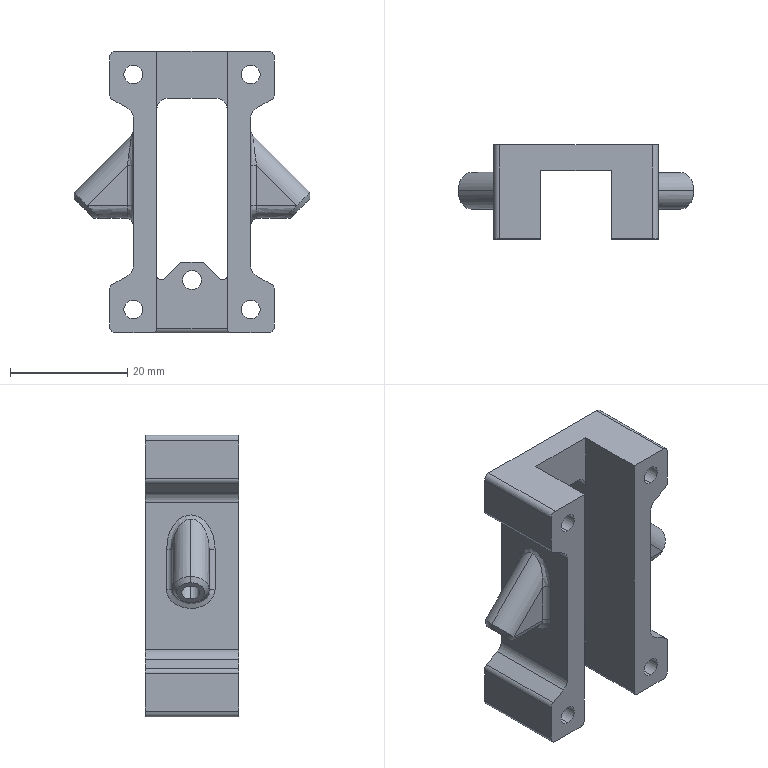Part | SolidWorks | features Fillet 4, ICE 4, MirrorPattern 2, Chamfer 1, Extrusion 1 | 1 solid | 84 faces | box 40.135 x 16 x 48 mm | volume 9698 mm3 | cylinder 43 | plane 31 | spline 6 | cone 4 | commonest cylinder face diameters 2 x14 3.2 x10 4 x6 1.5 x5 3.06 x4 6.26 x4